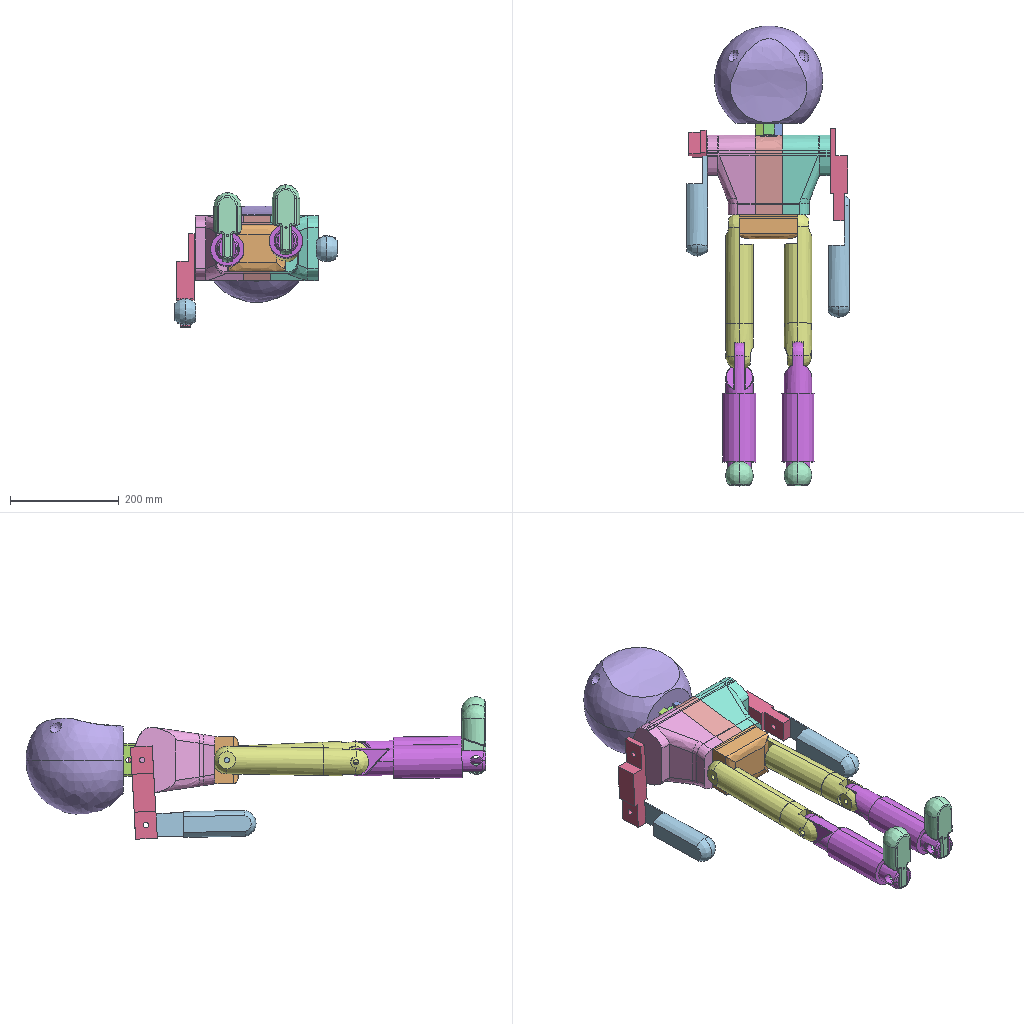Assembly | SolidWorks | 11 different items | 16 placed | box 299 x 848 x 263 mm
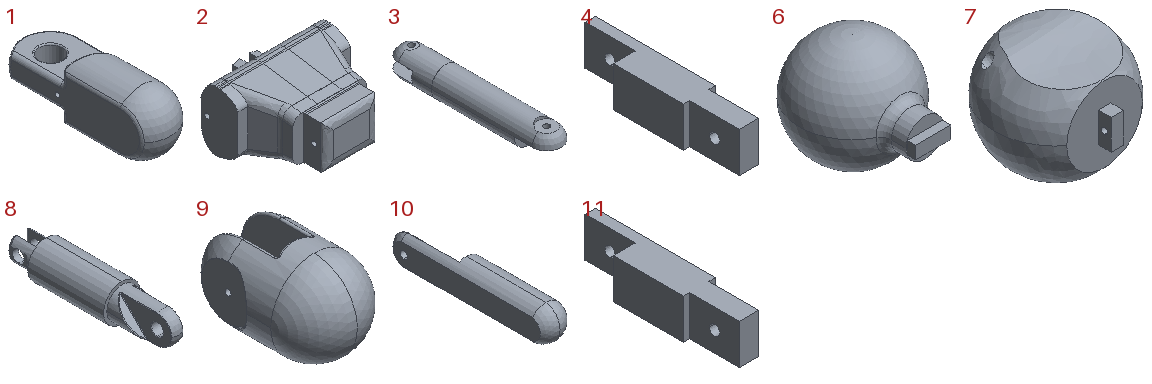Parts list (item | quantity | size | volume | features):
1 | x2 | 43.4 x 129 x 50.8 mm | 154558 mm3 | features ICE 7, Fillet 2, MirrorPattern 1, MoveCopyBody 1, Revolution 1, Scale 1
2 | x1 | 227 x 215.464 x 120.276 mm | 3397637 mm3 | features ICE 19, Fillet 4, MoveCopyBody 4, Revolution 2, Scale 2, Split 1
3 | x2 | 50.8 x 286.949 x 50.8 mm | 448364 mm3 | features ICE 10, Fillet 1, MoveCopyBody 1, Revolution 1, Scale 1, Split 1
4 | x2 | 31.854 x 170 x 40 mm | 145748 mm3 | features ICE 19, Fillet 2, MirrorPattern 1, Revolution 1, Scale 1
5 | x1 | - | - | -
6 | x1 | 218.44 x 273.05 x 218.44 mm | 5685357 mm3 | features ICE 4, Revolution 2, Fillet 1, Scale 1
7 | x1 | - | 3831189 mm3 | features ICE 7, MirrorPattern 1, RevCut 1, Revolution 1
8 | x2 | 61.465 x 264.6 x 61.465 mm | 508249 mm3 | features ICE 11, Fillet 2, MirrorPattern 1, MoveCopyBody 1, Revolution 1, Scale 1, Split 1
9 | x1 | 146.538 x 226.907 x 146.538 mm | 1909002 mm3 | features ICE 14, Fillet 4, Revolution 2, Scale 2
10 | x2 | 37.836 x 225.102 x 47.771 mm | 229671 mm3 | features ICE 12, Fillet 4, RevCut 1, Revolution 1, Scale 1
11 | x1 | 31.854 x 170 x 40 mm | 145748 mm3 | features ICE 19, Fillet 2, MirrorPattern 1, Revolution 1, Scale 1
Mates (type | each side: item.copy, entity, surface, feature):
Coincident | 2.1 face plane Boss-Extrude1-T | 7.1 face plane Boss-Extrude1
Coincident | 4.1 face plane Cut-Extrude9 | 10.1 face plane Cut-Extrude2
Concentric | 4.1 face cylinder Cut-Extrude10 | 10.1 face cylinder Boss-Extrude1
DistanceDim | 2.1 face plane Boss-Extrude3 | 4.1 face plane Cut-Extrude3
Coincident | 2.1 face plane Cut-Extrude5-T | 3.1 face plane Cut-Extrude4-T
Coincident | 3.1 face plane Cut-Extrude1 | 8.1 face plane Cut-Extrude2
Coincident | 8.1 face plane Cut-Extrude3-T | 1.1 face plane Cut-Extrude1
Concentric | 8.1 face cylinder Cut-Extrude1-T | 1.1 face cylinder Cut-Extrude3
Parallel | 8.1 face plane Cut-Extrude3-T | 1.1 face plane Cut-Extrude1-T
Concentric | 3.1 face cylinder Cut-Extrude3 | 8.1 face cylinder Cut-Extrude1-T
Coincident | 2.1 face cylinder Cut-Extrude9 | 4.1 edge
Parallel | 2.1 face plane Boss-Extrude1-T | 7.1 face plane Cut-Extrude5
Concentric | 2.1 face cylinder Cut-Extrude8 | 7.1 face cylinder Cut-Extrude3
Coincident | 2.1 face plane Boss-Extrude4 | 4.2 face plane Cut-Extrude3
Concentric | 2.1 face cylinder Cut-Extrude10 | 4.2 face cylinder Cut-Extrude5
Coincident | 4.2 face plane Cut-Extrude9 | 10.2 face plane Cut-Extrude2
Concentric | 4.2 face cylinder Cut-Extrude10 | 10.2 face cylinder Boss-Extrude1
Coincident | 2.1 face plane Cut-Extrude5-T | 3.2 face plane Cut-Extrude4-T
Coincident | 3.2 face plane Cut-Extrude1 | 8.2 face plane Cut-Extrude2
Concentric | 3.2 face cylinder Cut-Extrude3 | 8.2 face cylinder Cut-Extrude1-T
Coincident | 8.2 face plane Cut-Extrude3-T | 1.2 face plane Cut-Extrude1
Concentric | 8.2 face cylinder Cut-Extrude1-T | 1.2 face cylinder Cut-Extrude3
Parallel | 8.2 face plane Cut-Extrude3-T | 1.2 face plane Cut-Extrude1-T
Coincident | 1.1 face plane Cut-Extrude1-T | 1.2 face plane Cut-Extrude1-T
Concentric | 2.1 face cylinder Boss-Extrude6 | 3.2 face cylinder Boss-Extrude2
Concentric | 2.1 face cylinder Boss-Extrude6 | 3.1 face cylinder Boss-Extrude2